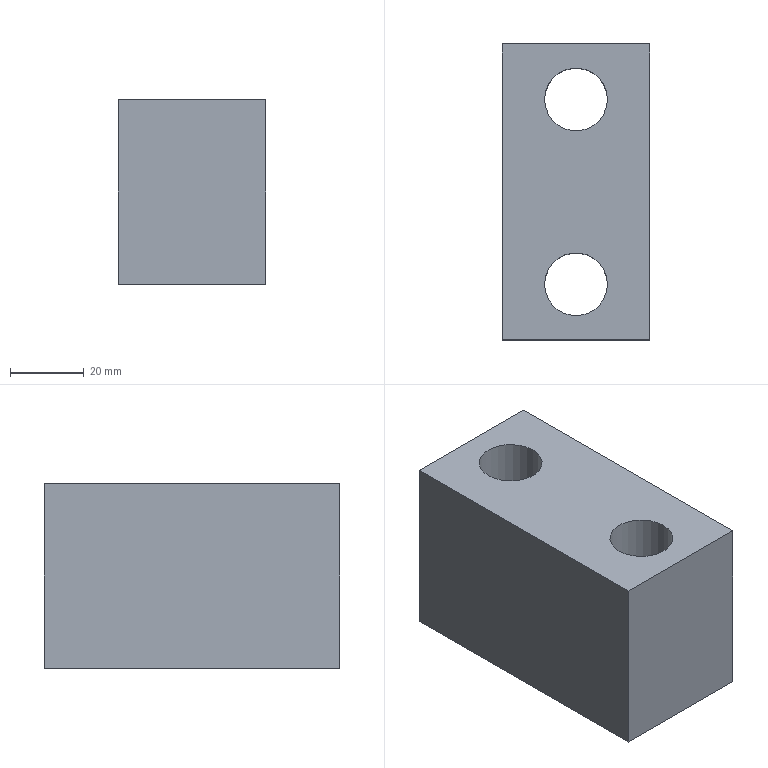Part | NX | features solid 2 | 1 solid | 8 faces | box 40 x 80 x 50 mm | volume 137302 mm3 | plane 6 | cylinder 2 | commonest cylinder face diameters 17 x2
STEP:
#1=CARTESIAN_POINT('',(775.,-165.,120.));
#2=VERTEX_POINT('',#1);
#3=CARTESIAN_POINT('',(775.,-245.,120.));
#4=VERTEX_POINT('',#3);
#5=CARTESIAN_POINT('',(775.,-270.,120.));
#6=DIRECTION('',(0.,-1.,0.));
#7=VECTOR('',#6,1000.);
#8=LINE('',#5,#7);
#9=EDGE_CURVE('',#2,#4,#8,.T.);
#10=ORIENTED_EDGE('',*,*,#9,.F.);
#11=CARTESIAN_POINT('',(775.,-165.,70.));
#12=VERTEX_POINT('',#11);
#13=CARTESIAN_POINT('',(775.,-165.,70.));
#14=DIRECTION('',(0.,0.,1.));
#15=VECTOR('',#14,1000.);
#16=LINE('',#13,#15);
#17=EDGE_CURVE('',#12,#2,#16,.T.);
#18=ORIENTED_EDGE('',*,*,#17,.F.);
#19=CARTESIAN_POINT('',(775.,-245.,70.));
#20=VERTEX_POINT('',#19);
#21=CARTESIAN_POINT('',(775.,-270.,70.));
#22=DIRECTION('',(0.,-1.,0.));
#23=VECTOR('',#22,1000.);
#24=LINE('',#21,#23);
#25=EDGE_CURVE('',#12,#20,#24,.T.);
#26=ORIENTED_EDGE('',*,*,#25,.T.);
#27=CARTESIAN_POINT('',(775.,-245.,70.));
#28=DIRECTION('',(0.,0.,1.));
#29=VECTOR('',#28,1000.);
#30=LINE('',#27,#29);
#31=EDGE_CURVE('',#20,#4,#30,.T.);
#32=ORIENTED_EDGE('',*,*,#31,.T.);
#33=EDGE_LOOP('',(#10,#18,#26,#32));
#34=FACE_BOUND('',#33,.T.);
#35=CARTESIAN_POINT('',(775.,-270.,70.));
#36=DIRECTION('',(-1.,0.,0.));
#37=DIRECTION('',(0.,-1.,0.));
#38=AXIS2_PLACEMENT_3D('',#35,#36,#37);
#39=PLANE('',#38);
#40=ADVANCED_FACE('',(#34),#39,.T.);
#41=CARTESIAN_POINT('',(815.,-245.,120.));
#42=VERTEX_POINT('',#41);
#43=CARTESIAN_POINT('',(780.,-245.,120.));
#44=DIRECTION('',(1.,0.,0.));
#45=VECTOR('',#44,1000.);
#46=LINE('',#43,#45);
#47=EDGE_CURVE('',#4,#42,#46,.T.);
#48=ORIENTED_EDGE('',*,*,#47,.F.);
#49=ORIENTED_EDGE('',*,*,#31,.F.);
#50=CARTESIAN_POINT('',(815.,-245.,70.));
#51=VERTEX_POINT('',#50);
#52=CARTESIAN_POINT('',(780.,-245.,70.));
#53=DIRECTION('',(1.,0.,0.));
#54=VECTOR('',#53,1000.);
#55=LINE('',#52,#54);
#56=EDGE_CURVE('',#20,#51,#55,.T.);
#57=ORIENTED_EDGE('',*,*,#56,.T.);
#58=CARTESIAN_POINT('',(815.,-245.,70.));
#59=DIRECTION('',(0.,0.,1.));
#60=VECTOR('',#59,1000.);
#61=LINE('',#58,#60);
#62=EDGE_CURVE('',#51,#42,#61,.T.);
#63=ORIENTED_EDGE('',*,*,#62,.T.);
#64=EDGE_LOOP('',(#48,#49,#57,#63));
#65=FACE_BOUND('',#64,.T.);
#66=CARTESIAN_POINT('',(780.,-245.,70.));
#67=DIRECTION('',(0.,-1.,0.));
#68=DIRECTION('',(0.,0.,-1.));
#69=AXIS2_PLACEMENT_3D('',#66,#67,#68);
#70=PLANE('',#69);
#71=ADVANCED_FACE('',(#65),#70,.T.);
#72=CARTESIAN_POINT('',(815.,-165.,120.));
#73=VERTEX_POINT('',#72);
#74=CARTESIAN_POINT('',(815.,-270.,120.));
#75=DIRECTION('',(0.,1.,0.));
#76=VECTOR('',#75,1000.);
#77=LINE('',#74,#76);
#78=EDGE_CURVE('',#42,#73,#77,.T.);
#79=ORIENTED_EDGE('',*,*,#78,.F.);
#80=ORIENTED_EDGE('',*,*,#62,.F.);
#81=CARTESIAN_POINT('',(815.,-165.,70.));
#82=VERTEX_POINT('',#81);
#83=CARTESIAN_POINT('',(815.,-270.,70.));
#84=DIRECTION('',(0.,1.,0.));
#85=VECTOR('',#84,1000.);
#86=LINE('',#83,#85);
#87=EDGE_CURVE('',#51,#82,#86,.T.);
#88=ORIENTED_EDGE('',*,*,#87,.T.);
#89=CARTESIAN_POINT('',(815.,-165.,70.));
#90=DIRECTION('',(0.,0.,1.));
#91=VECTOR('',#90,1000.);
#92=LINE('',#89,#91);
#93=EDGE_CURVE('',#82,#73,#92,.T.);
#94=ORIENTED_EDGE('',*,*,#93,.T.);
#95=EDGE_LOOP('',(#79,#80,#88,#94));
#96=FACE_BOUND('',#95,.T.);
#97=CARTESIAN_POINT('',(815.,-270.,70.));
#98=DIRECTION('',(1.,0.,0.));
#99=DIRECTION('',(0.,0.,-1.));
#100=AXIS2_PLACEMENT_3D('',#97,#98,#99);
#101=PLANE('',#100);
#102=ADVANCED_FACE('',(#96),#101,.T.);
#103=CARTESIAN_POINT('',(803.5,-230.,70.));
#104=VERTEX_POINT('',#103);
#105=CARTESIAN_POINT('',(795.,-230.,70.));
#106=DIRECTION('',(0.,0.,-1.));
#107=DIRECTION('',(1.,0.,0.));
#108=AXIS2_PLACEMENT_3D('',#105,#106,#107);
#109=CIRCLE('',#108,8.5);
#110=EDGE_CURVE('',#104,#104,#109,.T.);
#111=ORIENTED_EDGE('',*,*,#110,.T.);
#112=EDGE_LOOP('',(#111));
#113=FACE_BOUND('',#112,.T.);
#114=CARTESIAN_POINT('',(803.5,-230.,120.));
#115=VERTEX_POINT('',#114);
#116=CARTESIAN_POINT('',(795.,-230.,120.));
#117=DIRECTION('',(0.,0.,-1.));
#118=DIRECTION('',(1.,0.,0.));
#119=AXIS2_PLACEMENT_3D('',#116,#117,#118);
#120=CIRCLE('',#119,8.5);
#121=EDGE_CURVE('',#115,#115,#120,.T.);
#122=ORIENTED_EDGE('',*,*,#121,.F.);
#123=EDGE_LOOP('',(#122));
#124=FACE_BOUND('',#123,.T.);
#125=CARTESIAN_POINT('',(795.,-230.,70.));
#126=DIRECTION('',(0.,0.,1.));
#127=DIRECTION('',(1.,0.,0.));
#128=AXIS2_PLACEMENT_3D('',#125,#126,#127);
#129=CYLINDRICAL_SURFACE('',#128,8.5);
#130=ADVANCED_FACE('',(#113,#124),#129,.F.);
#131=CARTESIAN_POINT('',(803.5,-180.,70.));
#132=VERTEX_POINT('',#131);
#133=CARTESIAN_POINT('',(795.,-180.,70.));
#134=DIRECTION('',(0.,0.,-1.));
#135=DIRECTION('',(1.,0.,0.));
#136=AXIS2_PLACEMENT_3D('',#133,#134,#135);
#137=CIRCLE('',#136,8.5);
#138=EDGE_CURVE('',#132,#132,#137,.T.);
#139=ORIENTED_EDGE('',*,*,#138,.T.);
#140=EDGE_LOOP('',(#139));
#141=FACE_BOUND('',#140,.T.);
#142=CARTESIAN_POINT('',(803.5,-180.,120.));
#143=VERTEX_POINT('',#142);
#144=CARTESIAN_POINT('',(795.,-180.,120.));
#145=DIRECTION('',(0.,0.,-1.));
#146=DIRECTION('',(1.,0.,0.));
#147=AXIS2_PLACEMENT_3D('',#144,#145,#146);
#148=CIRCLE('',#147,8.5);
#149=EDGE_CURVE('',#143,#143,#148,.T.);
#150=ORIENTED_EDGE('',*,*,#149,.F.);
#151=EDGE_LOOP('',(#150));
#152=FACE_BOUND('',#151,.T.);
#153=CARTESIAN_POINT('',(795.,-180.,70.));
#154=DIRECTION('',(0.,0.,1.));
#155=DIRECTION('',(1.,0.,0.));
#156=AXIS2_PLACEMENT_3D('',#153,#154,#155);
#157=CYLINDRICAL_SURFACE('',#156,8.5);
#158=ADVANCED_FACE('',(#141,#152),#157,.F.);
#159=CARTESIAN_POINT('',(780.,-165.,120.));
#160=DIRECTION('',(-1.,0.,0.));
#161=VECTOR('',#160,1000.);
#162=LINE('',#159,#161);
#163=EDGE_CURVE('',#73,#2,#162,.T.);
#164=ORIENTED_EDGE('',*,*,#163,.F.);
#165=ORIENTED_EDGE('',*,*,#93,.F.);
#166=CARTESIAN_POINT('',(780.,-165.,70.));
#167=DIRECTION('',(-1.,0.,0.));
#168=VECTOR('',#167,1000.);
#169=LINE('',#166,#168);
#170=EDGE_CURVE('',#82,#12,#169,.T.);
#171=ORIENTED_EDGE('',*,*,#170,.T.);
#172=ORIENTED_EDGE('',*,*,#17,.T.);
#173=EDGE_LOOP('',(#164,#165,#171,#172));
#174=FACE_BOUND('',#173,.T.);
#175=CARTESIAN_POINT('',(780.,-165.,70.));
#176=DIRECTION('',(0.,1.,0.));
#177=DIRECTION('',(0.,0.,1.));
#178=AXIS2_PLACEMENT_3D('',#175,#176,#177);
#179=PLANE('',#178);
#180=ADVANCED_FACE('',(#174),#179,.T.);
#181=ORIENTED_EDGE('',*,*,#138,.F.);
#182=EDGE_LOOP('',(#181));
#183=FACE_BOUND('',#182,.T.);
#184=ORIENTED_EDGE('',*,*,#110,.F.);
#185=EDGE_LOOP('',(#184));
#186=FACE_BOUND('',#185,.T.);
#187=ORIENTED_EDGE('',*,*,#25,.F.);
#188=ORIENTED_EDGE('',*,*,#170,.F.);
#189=ORIENTED_EDGE('',*,*,#87,.F.);
#190=ORIENTED_EDGE('',*,*,#56,.F.);
#191=EDGE_LOOP('',(#187,#188,#189,#190));
#192=FACE_BOUND('',#191,.T.);
#193=CARTESIAN_POINT('',(780.,-270.,70.));
#194=DIRECTION('',(0.,0.,-1.));
#195=DIRECTION('',(1.,0.,0.));
#196=AXIS2_PLACEMENT_3D('',#193,#194,#195);
#197=PLANE('',#196);
#198=ADVANCED_FACE('',(#183,#186,#192),#197,.T.);
#199=ORIENTED_EDGE('',*,*,#149,.T.);
#200=EDGE_LOOP('',(#199));
#201=FACE_BOUND('',#200,.T.);
#202=ORIENTED_EDGE('',*,*,#121,.T.);
#203=EDGE_LOOP('',(#202));
#204=FACE_BOUND('',#203,.T.);
#205=ORIENTED_EDGE('',*,*,#9,.T.);
#206=ORIENTED_EDGE('',*,*,#47,.T.);
#207=ORIENTED_EDGE('',*,*,#78,.T.);
#208=ORIENTED_EDGE('',*,*,#163,.T.);
#209=EDGE_LOOP('',(#205,#206,#207,#208));
#210=FACE_BOUND('',#209,.T.);
#211=CARTESIAN_POINT('',(780.,-270.,120.));
#212=DIRECTION('',(0.,0.,-1.));
#213=DIRECTION('',(1.,0.,0.));
#214=AXIS2_PLACEMENT_3D('',#211,#212,#213);
#215=PLANE('',#214);
#216=ADVANCED_FACE('',(#201,#204,#210),#215,.F.);
#217=CLOSED_SHELL('',(#40,#71,#102,#130,#158,#180,#198,#216));
#218=MANIFOLD_SOLID_BREP('',#217);
#219=(LENGTH_UNIT()NAMED_UNIT(*)SI_UNIT(.MILLI.,.METRE.));
#220=UNCERTAINTY_MEASURE_WITH_UNIT(LENGTH_MEASURE(0.00001),#219,'','');
#221=(NAMED_UNIT(*)PLANE_ANGLE_UNIT()SI_UNIT($,.RADIAN.));
#222=(NAMED_UNIT(*)SI_UNIT($,.STERADIAN.)SOLID_ANGLE_UNIT());
#223=(GEOMETRIC_REPRESENTATION_CONTEXT(3)GLOBAL_UNCERTAINTY_ASSIGNED_CONTEXT((#220))GLOBAL_UNIT_ASSIGNED_CONTEXT((#219,#221,#222))REPRESENTATION_CONTEXT('',''));
#224=ADVANCED_BREP_SHAPE_REPRESENTATION('',(#218),#223);